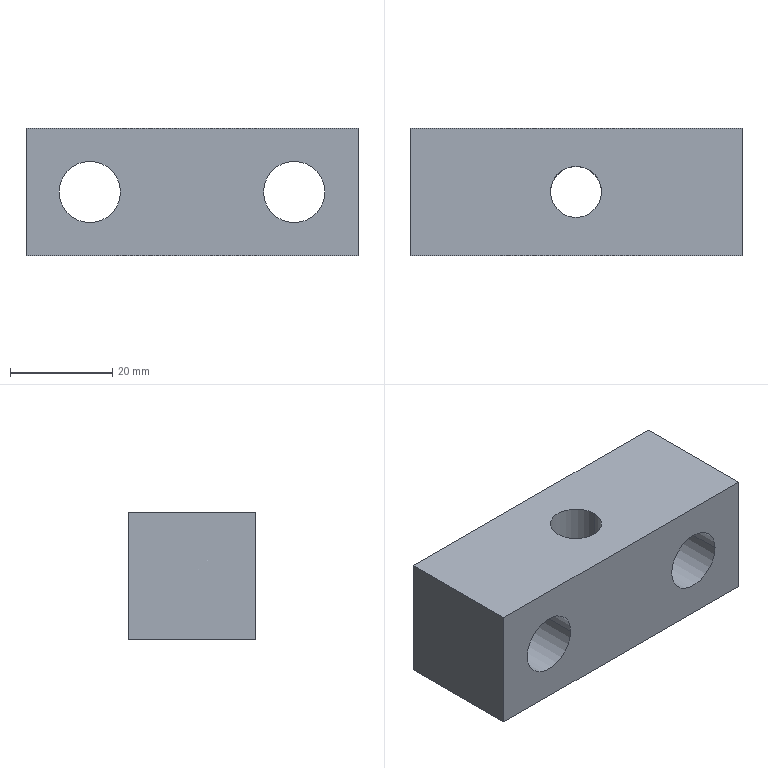Part | STEP file | J452-EBZ05-21-04-Part-1 | 1 solid | 12 faces | box 65 x 25 x 25 mm | volume 33007 mm3 | cylinder 6 | plane 6 | commonest cylinder face diameters 12 x4 10 x2
STEP:
#1=CARTESIAN_POINT('',(0.,0.,0.));
#2=DIRECTION('',(0.,0.,1.));
#3=DIRECTION('',(1.,0.,0.));
#4=AXIS2_PLACEMENT_3D('',#1,#2,#3);
#5=CARTESIAN_POINT('',(27.5,12.5,25.));
#6=VERTEX_POINT('',#5);
#7=CARTESIAN_POINT('',(27.5,12.5,0.));
#8=VERTEX_POINT('',#7);
#9=CARTESIAN_POINT('',(27.5,12.5,25.));
#10=DIRECTION('',(0.,0.,-1.));
#11=VECTOR('',#10,1.);
#12=LINE('',#9,#11);
#13=CARTESIAN_POINT('',(32.5,12.5,25.));
#14=DIRECTION('',(0.,0.,-1.));
#15=DIRECTION('',(-1.,0.,0.));
#16=AXIS2_PLACEMENT_3D('',#13,#14,#15);
#17=CYLINDRICAL_SURFACE('',#16,5.);
#18=CARTESIAN_POINT('',(6.283,0.));
#19=DIRECTION('',(0.,1.));
#20=VECTOR('',#19,1.);
#21=LINE('',#18,#20);
#22=(GEOMETRIC_REPRESENTATION_CONTEXT(2)PARAMETRIC_REPRESENTATION_CONTEXT()REPRESENTATION_CONTEXT('',''));
#23=DEFINITIONAL_REPRESENTATION('',(#21),#22);
#24=PCURVE('',#17,#23);
#25=CARTESIAN_POINT('',(32.5,12.5,25.));
#26=DIRECTION('',(0.,0.,-1.));
#27=DIRECTION('',(-1.,0.,0.));
#28=AXIS2_PLACEMENT_3D('',#25,#26,#27);
#29=CYLINDRICAL_SURFACE('',#28,5.);
#30=CARTESIAN_POINT('',(0.,0.));
#31=DIRECTION('',(0.,1.));
#32=VECTOR('',#31,1.);
#33=LINE('',#30,#32);
#34=(GEOMETRIC_REPRESENTATION_CONTEXT(2)PARAMETRIC_REPRESENTATION_CONTEXT()REPRESENTATION_CONTEXT('',''));
#35=DEFINITIONAL_REPRESENTATION('',(#33),#34);
#36=PCURVE('',#29,#35);
#37=SURFACE_CURVE('',#12,(#24,#36),.PCURVE_S1.);
#38=EDGE_CURVE('',#6,#8,#37,.T.);
#39=ORIENTED_EDGE('',*,*,#38,.T.);
#40=CARTESIAN_POINT('',(37.5,12.5,0.));
#41=VERTEX_POINT('',#40);
#42=CARTESIAN_POINT('',(32.5,12.5,0.));
#43=DIRECTION('',(0.,0.,1.));
#44=DIRECTION('',(1.,0.,0.));
#45=AXIS2_PLACEMENT_3D('',#42,#43,#44);
#46=CIRCLE('',#45,5.);
#47=CARTESIAN_POINT('',(9.425,25.));
#48=DIRECTION('',(-1.,0.));
#49=VECTOR('',#48,1.);
#50=LINE('',#47,#49);
#51=(GEOMETRIC_REPRESENTATION_CONTEXT(2)PARAMETRIC_REPRESENTATION_CONTEXT()REPRESENTATION_CONTEXT('',''));
#52=DEFINITIONAL_REPRESENTATION('',(#50),#51);
#53=PCURVE('',#17,#52);
#54=CARTESIAN_POINT('',(0.,12.5,0.));
#55=DIRECTION('',(0.,0.,-1.));
#56=DIRECTION('',(-1.,0.,0.));
#57=AXIS2_PLACEMENT_3D('',#54,#55,#56);
#58=PLANE('',#57);
#59=CARTESIAN_POINT('',(-37.5,0.));
#60=CARTESIAN_POINT('',(-37.5,8.66));
#61=CARTESIAN_POINT('',(-30.,4.33));
#62=CARTESIAN_POINT('',(-22.5,0.));
#63=CARTESIAN_POINT('',(-30.,-4.33));
#64=CARTESIAN_POINT('',(-37.5,-8.66));
#65=CARTESIAN_POINT('',(-37.5,0.));
#66=(BOUNDED_CURVE()B_SPLINE_CURVE(2,(#59,#60,#61,#62,#63,#64,#65),.UNSPECIFIED.,.T.,.F.)B_SPLINE_CURVE_WITH_KNOTS((1,2,2,2,2,1),(-2.094,0.,2.094,4.189,6.283,8.378),.UNSPECIFIED.)CURVE()GEOMETRIC_REPRESENTATION_ITEM()RATIONAL_B_SPLINE_CURVE((1.,0.5,1.,0.5,1.,0.5,1.))REPRESENTATION_ITEM(''));
#67=(GEOMETRIC_REPRESENTATION_CONTEXT(2)PARAMETRIC_REPRESENTATION_CONTEXT()REPRESENTATION_CONTEXT('',''));
#68=DEFINITIONAL_REPRESENTATION('',(#66),#67);
#69=PCURVE('',#58,#68);
#70=SURFACE_CURVE('',#46,(#53,#69),.PCURVE_S1.);
#71=EDGE_CURVE('',#8,#41,#70,.T.);
#72=ORIENTED_EDGE('',*,*,#71,.T.);
#73=CARTESIAN_POINT('',(37.5,12.5,25.));
#74=VERTEX_POINT('',#73);
#75=CARTESIAN_POINT('',(37.5,12.5,25.));
#76=DIRECTION('',(0.,0.,-1.));
#77=VECTOR('',#76,1.);
#78=LINE('',#75,#77);
#79=CARTESIAN_POINT('',(3.142,0.));
#80=DIRECTION('',(0.,1.));
#81=VECTOR('',#80,1.);
#82=LINE('',#79,#81);
#83=(GEOMETRIC_REPRESENTATION_CONTEXT(2)PARAMETRIC_REPRESENTATION_CONTEXT()REPRESENTATION_CONTEXT('',''));
#84=DEFINITIONAL_REPRESENTATION('',(#82),#83);
#85=PCURVE('',#17,#84);
#86=CARTESIAN_POINT('',(3.142,0.));
#87=DIRECTION('',(0.,1.));
#88=VECTOR('',#87,1.);
#89=LINE('',#86,#88);
#90=(GEOMETRIC_REPRESENTATION_CONTEXT(2)PARAMETRIC_REPRESENTATION_CONTEXT()REPRESENTATION_CONTEXT('',''));
#91=DEFINITIONAL_REPRESENTATION('',(#89),#90);
#92=PCURVE('',#29,#91);
#93=SURFACE_CURVE('',#78,(#85,#92),.PCURVE_S1.);
#94=EDGE_CURVE('',#74,#41,#93,.T.);
#95=ORIENTED_EDGE('',*,*,#94,.F.);
#96=CARTESIAN_POINT('',(32.5,12.5,25.));
#97=DIRECTION('',(0.,0.,-1.));
#98=DIRECTION('',(-1.,0.,0.));
#99=AXIS2_PLACEMENT_3D('',#96,#97,#98);
#100=CIRCLE('',#99,5.);
#101=CARTESIAN_POINT('',(0.,0.));
#102=DIRECTION('',(1.,0.));
#103=VECTOR('',#102,1.);
#104=LINE('',#101,#103);
#105=(GEOMETRIC_REPRESENTATION_CONTEXT(2)PARAMETRIC_REPRESENTATION_CONTEXT()REPRESENTATION_CONTEXT('',''));
#106=DEFINITIONAL_REPRESENTATION('',(#104),#105);
#107=PCURVE('',#17,#106);
#108=CARTESIAN_POINT('',(0.,12.5,25.));
#109=DIRECTION('',(0.,0.,1.));
#110=DIRECTION('',(1.,0.,0.));
#111=AXIS2_PLACEMENT_3D('',#108,#109,#110);
#112=PLANE('',#111);
#113=CARTESIAN_POINT('',(27.5,0.));
#114=CARTESIAN_POINT('',(27.5,8.66));
#115=CARTESIAN_POINT('',(35.,4.33));
#116=CARTESIAN_POINT('',(42.5,0.));
#117=CARTESIAN_POINT('',(35.,-4.33));
#118=CARTESIAN_POINT('',(27.5,-8.66));
#119=CARTESIAN_POINT('',(27.5,0.));
#120=(BOUNDED_CURVE()B_SPLINE_CURVE(2,(#113,#114,#115,#116,#117,#118,#119),.UNSPECIFIED.,.T.,.F.)B_SPLINE_CURVE_WITH_KNOTS((1,2,2,2,2,1),(-2.094,0.,2.094,4.189,6.283,8.378),.UNSPECIFIED.)CURVE()GEOMETRIC_REPRESENTATION_ITEM()RATIONAL_B_SPLINE_CURVE((1.,0.5,1.,0.5,1.,0.5,1.))REPRESENTATION_ITEM(''));
#121=(GEOMETRIC_REPRESENTATION_CONTEXT(2)PARAMETRIC_REPRESENTATION_CONTEXT()REPRESENTATION_CONTEXT('',''));
#122=DEFINITIONAL_REPRESENTATION('',(#120),#121);
#123=PCURVE('',#112,#122);
#124=SURFACE_CURVE('',#100,(#107,#123),.PCURVE_S1.);
#125=EDGE_CURVE('',#74,#6,#124,.T.);
#126=ORIENTED_EDGE('',*,*,#125,.T.);
#127=EDGE_LOOP('',(#39,#72,#95,#126));
#128=FACE_BOUND('',#127,.F.);
#129=ADVANCED_FACE('',(#128),#17,.F.);
#130=CARTESIAN_POINT('',(46.5,0.,12.5));
#131=VERTEX_POINT('',#130);
#132=CARTESIAN_POINT('',(46.5,25.,12.5));
#133=VERTEX_POINT('',#132);
#134=CARTESIAN_POINT('',(46.5,0.,12.5));
#135=DIRECTION('',(0.,1.,0.));
#136=VECTOR('',#135,1.);
#137=LINE('',#134,#136);
#138=CARTESIAN_POINT('',(52.5,0.,12.5));
#139=DIRECTION('',(0.,1.,0.));
#140=DIRECTION('',(-1.,0.,0.));
#141=AXIS2_PLACEMENT_3D('',#138,#139,#140);
#142=CYLINDRICAL_SURFACE('',#141,6.);
#143=CARTESIAN_POINT('',(6.283,0.));
#144=DIRECTION('',(0.,1.));
#145=VECTOR('',#144,1.);
#146=LINE('',#143,#145);
#147=(GEOMETRIC_REPRESENTATION_CONTEXT(2)PARAMETRIC_REPRESENTATION_CONTEXT()REPRESENTATION_CONTEXT('',''));
#148=DEFINITIONAL_REPRESENTATION('',(#146),#147);
#149=PCURVE('',#142,#148);
#150=CARTESIAN_POINT('',(52.5,0.,12.5));
#151=DIRECTION('',(0.,1.,0.));
#152=DIRECTION('',(-1.,0.,0.));
#153=AXIS2_PLACEMENT_3D('',#150,#151,#152);
#154=CYLINDRICAL_SURFACE('',#153,6.);
#155=CARTESIAN_POINT('',(0.,0.));
#156=DIRECTION('',(0.,1.));
#157=VECTOR('',#156,1.);
#158=LINE('',#155,#157);
#159=(GEOMETRIC_REPRESENTATION_CONTEXT(2)PARAMETRIC_REPRESENTATION_CONTEXT()REPRESENTATION_CONTEXT('',''));
#160=DEFINITIONAL_REPRESENTATION('',(#158),#159);
#161=PCURVE('',#154,#160);
#162=SURFACE_CURVE('',#137,(#149,#161),.PCURVE_S1.);
#163=EDGE_CURVE('',#131,#133,#162,.T.);
#164=ORIENTED_EDGE('',*,*,#163,.T.);
#165=CARTESIAN_POINT('',(58.5,25.,12.5));
#166=VERTEX_POINT('',#165);
#167=CARTESIAN_POINT('',(52.5,25.,12.5));
#168=DIRECTION('',(0.,-1.,0.));
#169=DIRECTION('',(1.,0.,0.));
#170=AXIS2_PLACEMENT_3D('',#167,#168,#169);
#171=CIRCLE('',#170,6.);
#172=CARTESIAN_POINT('',(9.425,25.));
#173=DIRECTION('',(-1.,0.));
#174=VECTOR('',#173,1.);
#175=LINE('',#172,#174);
#176=(GEOMETRIC_REPRESENTATION_CONTEXT(2)PARAMETRIC_REPRESENTATION_CONTEXT()REPRESENTATION_CONTEXT('',''));
#177=DEFINITIONAL_REPRESENTATION('',(#175),#176);
#178=PCURVE('',#142,#177);
#179=CARTESIAN_POINT('',(0.,25.,12.5));
#180=DIRECTION('',(0.,1.,0.));
#181=DIRECTION('',(-1.,0.,0.));
#182=AXIS2_PLACEMENT_3D('',#179,#180,#181);
#183=PLANE('',#182);
#184=CARTESIAN_POINT('',(-58.5,0.));
#185=CARTESIAN_POINT('',(-58.5,10.392));
#186=CARTESIAN_POINT('',(-49.5,5.196));
#187=CARTESIAN_POINT('',(-40.5,0.));
#188=CARTESIAN_POINT('',(-49.5,-5.196));
#189=CARTESIAN_POINT('',(-58.5,-10.392));
#190=CARTESIAN_POINT('',(-58.5,0.));
#191=(BOUNDED_CURVE()B_SPLINE_CURVE(2,(#184,#185,#186,#187,#188,#189,#190),.UNSPECIFIED.,.T.,.F.)B_SPLINE_CURVE_WITH_KNOTS((1,2,2,2,2,1),(-2.094,0.,2.094,4.189,6.283,8.378),.UNSPECIFIED.)CURVE()GEOMETRIC_REPRESENTATION_ITEM()RATIONAL_B_SPLINE_CURVE((1.,0.5,1.,0.5,1.,0.5,1.))REPRESENTATION_ITEM(''));
#192=(GEOMETRIC_REPRESENTATION_CONTEXT(2)PARAMETRIC_REPRESENTATION_CONTEXT()REPRESENTATION_CONTEXT('',''));
#193=DEFINITIONAL_REPRESENTATION('',(#191),#192);
#194=PCURVE('',#183,#193);
#195=SURFACE_CURVE('',#171,(#178,#194),.PCURVE_S1.);
#196=EDGE_CURVE('',#133,#166,#195,.T.);
#197=ORIENTED_EDGE('',*,*,#196,.T.);
#198=CARTESIAN_POINT('',(58.5,0.,12.5));
#199=VERTEX_POINT('',#198);
#200=CARTESIAN_POINT('',(58.5,0.,12.5));
#201=DIRECTION('',(0.,1.,0.));
#202=VECTOR('',#201,1.);
#203=LINE('',#200,#202);
#204=CARTESIAN_POINT('',(3.142,0.));
#205=DIRECTION('',(0.,1.));
#206=VECTOR('',#205,1.);
#207=LINE('',#204,#206);
#208=(GEOMETRIC_REPRESENTATION_CONTEXT(2)PARAMETRIC_REPRESENTATION_CONTEXT()REPRESENTATION_CONTEXT('',''));
#209=DEFINITIONAL_REPRESENTATION('',(#207),#208);
#210=PCURVE('',#142,#209);
#211=CARTESIAN_POINT('',(3.142,0.));
#212=DIRECTION('',(0.,1.));
#213=VECTOR('',#212,1.);
#214=LINE('',#211,#213);
#215=(GEOMETRIC_REPRESENTATION_CONTEXT(2)PARAMETRIC_REPRESENTATION_CONTEXT()REPRESENTATION_CONTEXT('',''));
#216=DEFINITIONAL_REPRESENTATION('',(#214),#215);
#217=PCURVE('',#154,#216);
#218=SURFACE_CURVE('',#203,(#210,#217),.PCURVE_S1.);
#219=EDGE_CURVE('',#199,#166,#218,.T.);
#220=ORIENTED_EDGE('',*,*,#219,.F.);
#221=CARTESIAN_POINT('',(52.5,0.,12.5));
#222=DIRECTION('',(0.,1.,0.));
#223=DIRECTION('',(-1.,0.,0.));
#224=AXIS2_PLACEMENT_3D('',#221,#222,#223);
#225=CIRCLE('',#224,6.);
#226=CARTESIAN_POINT('',(0.,0.));
#227=DIRECTION('',(1.,0.));
#228=VECTOR('',#227,1.);
#229=LINE('',#226,#228);
#230=(GEOMETRIC_REPRESENTATION_CONTEXT(2)PARAMETRIC_REPRESENTATION_CONTEXT()REPRESENTATION_CONTEXT('',''));
#231=DEFINITIONAL_REPRESENTATION('',(#229),#230);
#232=PCURVE('',#142,#231);
#233=CARTESIAN_POINT('',(0.,0.,12.5));
#234=DIRECTION('',(0.,-1.,0.));
#235=DIRECTION('',(1.,0.,0.));
#236=AXIS2_PLACEMENT_3D('',#233,#234,#235);
#237=PLANE('',#236);
#238=CARTESIAN_POINT('',(46.5,0.));
#239=CARTESIAN_POINT('',(46.5,10.392));
#240=CARTESIAN_POINT('',(55.5,5.196));
#241=CARTESIAN_POINT('',(64.5,0.));
#242=CARTESIAN_POINT('',(55.5,-5.196));
#243=CARTESIAN_POINT('',(46.5,-10.392));
#244=CARTESIAN_POINT('',(46.5,0.));
#245=(BOUNDED_CURVE()B_SPLINE_CURVE(2,(#238,#239,#240,#241,#242,#243,#244),.UNSPECIFIED.,.T.,.F.)B_SPLINE_CURVE_WITH_KNOTS((1,2,2,2,2,1),(-2.094,0.,2.094,4.189,6.283,8.378),.UNSPECIFIED.)CURVE()GEOMETRIC_REPRESENTATION_ITEM()RATIONAL_B_SPLINE_CURVE((1.,0.5,1.,0.5,1.,0.5,1.))REPRESENTATION_ITEM(''));
#246=(GEOMETRIC_REPRESENTATION_CONTEXT(2)PARAMETRIC_REPRESENTATION_CONTEXT()REPRESENTATION_CONTEXT('',''));
#247=DEFINITIONAL_REPRESENTATION('',(#245),#246);
#248=PCURVE('',#237,#247);
#249=SURFACE_CURVE('',#225,(#232,#248),.PCURVE_S1.);
#250=EDGE_CURVE('',#199,#131,#249,.T.);
#251=ORIENTED_EDGE('',*,*,#250,.T.);
#252=EDGE_LOOP('',(#164,#197,#220,#251));
#253=FACE_BOUND('',#252,.F.);
#254=ADVANCED_FACE('',(#253),#142,.F.);
#255=CARTESIAN_POINT('',(6.5,0.,12.5));
#256=VERTEX_POINT('',#255);
#257=CARTESIAN_POINT('',(6.5,25.,12.5));
#258=VERTEX_POINT('',#257);
#259=CARTESIAN_POINT('',(6.5,0.,12.5));
#260=DIRECTION('',(0.,1.,0.));
#261=VECTOR('',#260,1.);
#262=LINE('',#259,#261);
#263=CARTESIAN_POINT('',(12.5,0.,12.5));
#264=DIRECTION('',(0.,1.,0.));
#265=DIRECTION('',(-1.,0.,0.));
#266=AXIS2_PLACEMENT_3D('',#263,#264,#265);
#267=CYLINDRICAL_SURFACE('',#266,6.);
#268=CARTESIAN_POINT('',(6.283,0.));
#269=DIRECTION('',(0.,1.));
#270=VECTOR('',#269,1.);
#271=LINE('',#268,#270);
#272=(GEOMETRIC_REPRESENTATION_CONTEXT(2)PARAMETRIC_REPRESENTATION_CONTEXT()REPRESENTATION_CONTEXT('',''));
#273=DEFINITIONAL_REPRESENTATION('',(#271),#272);
#274=PCURVE('',#267,#273);
#275=CARTESIAN_POINT('',(12.5,0.,12.5));
#276=DIRECTION('',(0.,1.,0.));
#277=DIRECTION('',(-1.,0.,0.));
#278=AXIS2_PLACEMENT_3D('',#275,#276,#277);
#279=CYLINDRICAL_SURFACE('',#278,6.);
#280=CARTESIAN_POINT('',(0.,0.));
#281=DIRECTION('',(0.,1.));
#282=VECTOR('',#281,1.);
#283=LINE('',#280,#282);
#284=(GEOMETRIC_REPRESENTATION_CONTEXT(2)PARAMETRIC_REPRESENTATION_CONTEXT()REPRESENTATION_CONTEXT('',''));
#285=DEFINITIONAL_REPRESENTATION('',(#283),#284);
#286=PCURVE('',#279,#285);
#287=SURFACE_CURVE('',#262,(#274,#286),.PCURVE_S1.);
#288=EDGE_CURVE('',#256,#258,#287,.T.);
#289=ORIENTED_EDGE('',*,*,#288,.T.);
#290=CARTESIAN_POINT('',(18.5,25.,12.5));
#291=VERTEX_POINT('',#290);
#292=CARTESIAN_POINT('',(12.5,25.,12.5));
#293=DIRECTION('',(0.,-1.,0.));
#294=DIRECTION('',(1.,0.,0.));
#295=AXIS2_PLACEMENT_3D('',#292,#293,#294);
#296=CIRCLE('',#295,6.);
#297=CARTESIAN_POINT('',(9.425,25.));
#298=DIRECTION('',(-1.,0.));
#299=VECTOR('',#298,1.);
#300=LINE('',#297,#299);
#301=(GEOMETRIC_REPRESENTATION_CONTEXT(2)PARAMETRIC_REPRESENTATION_CONTEXT()REPRESENTATION_CONTEXT('',''));
#302=DEFINITIONAL_REPRESENTATION('',(#300),#301);
#303=PCURVE('',#267,#302);
#304=CARTESIAN_POINT('',(-18.5,0.));
#305=CARTESIAN_POINT('',(-18.5,10.392));
#306=CARTESIAN_POINT('',(-9.5,5.196));
#307=CARTESIAN_POINT('',(-0.5,0.));
#308=CARTESIAN_POINT('',(-9.5,-5.196));
#309=CARTESIAN_POINT('',(-18.5,-10.392));
#310=CARTESIAN_POINT('',(-18.5,0.));
#311=(BOUNDED_CURVE()B_SPLINE_CURVE(2,(#304,#305,#306,#307,#308,#309,#310),.UNSPECIFIED.,.T.,.F.)B_SPLINE_CURVE_WITH_KNOTS((1,2,2,2,2,1),(-2.094,0.,2.094,4.189,6.283,8.378),.UNSPECIFIED.)CURVE()GEOMETRIC_REPRESENTATION_ITEM()RATIONAL_B_SPLINE_CURVE((1.,0.5,1.,0.5,1.,0.5,1.))REPRESENTATION_ITEM(''));
#312=(GEOMETRIC_REPRESENTATION_CONTEXT(2)PARAMETRIC_REPRESENTATION_CONTEXT()REPRESENTATION_CONTEXT('',''));
#313=DEFINITIONAL_REPRESENTATION('',(#311),#312);
#314=PCURVE('',#183,#313);
#315=SURFACE_CURVE('',#296,(#303,#314),.PCURVE_S1.);
#316=EDGE_CURVE('',#258,#291,#315,.T.);
#317=ORIENTED_EDGE('',*,*,#316,.T.);
#318=CARTESIAN_POINT('',(18.5,0.,12.5));
#319=VERTEX_POINT('',#318);
#320=CARTESIAN_POINT('',(18.5,0.,12.5));
#321=DIRECTION('',(0.,1.,0.));
#322=VECTOR('',#321,1.);
#323=LINE('',#320,#322);
#324=CARTESIAN_POINT('',(3.142,0.));
#325=DIRECTION('',(0.,1.));
#326=VECTOR('',#325,1.);
#327=LINE('',#324,#326);
#328=(GEOMETRIC_REPRESENTATION_CONTEXT(2)PARAMETRIC_REPRESENTATION_CONTEXT()REPRESENTATION_CONTEXT('',''));
#329=DEFINITIONAL_REPRESENTATION('',(#327),#328);
#330=PCURVE('',#267,#329);
#331=CARTESIAN_POINT('',(3.142,0.));
#332=DIRECTION('',(0.,1.));
#333=VECTOR('',#332,1.);
#334=LINE('',#331,#333);
#335=(GEOMETRIC_REPRESENTATION_CONTEXT(2)PARAMETRIC_REPRESENTATION_CONTEXT()REPRESENTATION_CONTEXT('',''));
#336=DEFINITIONAL_REPRESENTATION('',(#334),#335);
#337=PCURVE('',#279,#336);
#338=SURFACE_CURVE('',#323,(#330,#337),.PCURVE_S1.);
#339=EDGE_CURVE('',#319,#291,#338,.T.);
#340=ORIENTED_EDGE('',*,*,#339,.F.);
#341=CARTESIAN_POINT('',(12.5,0.,12.5));
#342=DIRECTION('',(0.,1.,0.));
#343=DIRECTION('',(-1.,0.,0.));
#344=AXIS2_PLACEMENT_3D('',#341,#342,#343);
#345=CIRCLE('',#344,6.);
#346=CARTESIAN_POINT('',(0.,0.));
#347=DIRECTION('',(1.,0.));
#348=VECTOR('',#347,1.);
#349=LINE('',#346,#348);
#350=(GEOMETRIC_REPRESENTATION_CONTEXT(2)PARAMETRIC_REPRESENTATION_CONTEXT()REPRESENTATION_CONTEXT('',''));
#351=DEFINITIONAL_REPRESENTATION('',(#349),#350);
#352=PCURVE('',#267,#351);
#353=CARTESIAN_POINT('',(6.5,0.));
#354=CARTESIAN_POINT('',(6.5,10.392));
#355=CARTESIAN_POINT('',(15.5,5.196));
#356=CARTESIAN_POINT('',(24.5,0.));
#357=CARTESIAN_POINT('',(15.5,-5.196));
#358=CARTESIAN_POINT('',(6.5,-10.392));
#359=CARTESIAN_POINT('',(6.5,0.));
#360=(BOUNDED_CURVE()B_SPLINE_CURVE(2,(#353,#354,#355,#356,#357,#358,#359),.UNSPECIFIED.,.T.,.F.)B_SPLINE_CURVE_WITH_KNOTS((1,2,2,2,2,1),(-2.094,0.,2.094,4.189,6.283,8.378),.UNSPECIFIED.)CURVE()GEOMETRIC_REPRESENTATION_ITEM()RATIONAL_B_SPLINE_CURVE((1.,0.5,1.,0.5,1.,0.5,1.))REPRESENTATION_ITEM(''));
#361=(GEOMETRIC_REPRESENTATION_CONTEXT(2)PARAMETRIC_REPRESENTATION_CONTEXT()REPRESENTATION_CONTEXT('',''));
#362=DEFINITIONAL_REPRESENTATION('',(#360),#361);
#363=PCURVE('',#237,#362);
#364=SURFACE_CURVE('',#345,(#352,#363),.PCURVE_S1.);
#365=EDGE_CURVE('',#319,#256,#364,.T.);
#366=ORIENTED_EDGE('',*,*,#365,.T.);
#367=EDGE_LOOP('',(#289,#317,#340,#366));
#368=FACE_BOUND('',#367,.F.);
#369=ADVANCED_FACE('',(#368),#267,.F.);
#370=CARTESIAN_POINT('',(65.,25.,0.));
#371=VERTEX_POINT('',#370);
#372=CARTESIAN_POINT('',(65.,0.,0.));
#373=VERTEX_POINT('',#372);
#374=CARTESIAN_POINT('',(65.,12.5,0.));
#375=DIRECTION('',(0.,-1.,0.));
#376=VECTOR('',#375,1.);
#377=LINE('',#374,#376);
#378=CARTESIAN_POINT('',(65.,12.5,12.5));
#379=DIRECTION('',(1.,0.,0.));
#380=DIRECTION('',(0.,1.,0.));
#381=AXIS2_PLACEMENT_3D('',#378,#379,#380);
#382=PLANE('',#381);
#383=CARTESIAN_POINT('',(0.,-12.5));
#384=DIRECTION('',(-1.,0.));
#385=VECTOR('',#384,1.);
#386=LINE('',#383,#385);
#387=(GEOMETRIC_REPRESENTATION_CONTEXT(2)PARAMETRIC_REPRESENTATION_CONTEXT()REPRESENTATION_CONTEXT('',''));
#388=DEFINITIONAL_REPRESENTATION('',(#386),#387);
#389=PCURVE('',#382,#388);
#390=CARTESIAN_POINT('',(-65.,0.));
#391=DIRECTION('',(0.,-1.));
#392=VECTOR('',#391,1.);
#393=LINE('',#390,#392);
#394=(GEOMETRIC_REPRESENTATION_CONTEXT(2)PARAMETRIC_REPRESENTATION_CONTEXT()REPRESENTATION_CONTEXT('',''));
#395=DEFINITIONAL_REPRESENTATION('',(#393),#394);
#396=PCURVE('',#58,#395);
#397=SURFACE_CURVE('',#377,(#389,#396),.PCURVE_S1.);
#398=EDGE_CURVE('',#371,#373,#397,.T.);
#399=ORIENTED_EDGE('',*,*,#398,.F.);
#400=CARTESIAN_POINT('',(65.,25.,25.));
#401=VERTEX_POINT('',#400);
#402=CARTESIAN_POINT('',(65.,25.,12.5));
#403=DIRECTION('',(0.,0.,-1.));
#404=VECTOR('',#403,1.);
#405=LINE('',#402,#404);
#406=CARTESIAN_POINT('',(12.5,0.));
#407=DIRECTION('',(0.,-1.));
#408=VECTOR('',#407,1.);
#409=LINE('',#406,#408);
#410=(GEOMETRIC_REPRESENTATION_CONTEXT(2)PARAMETRIC_REPRESENTATION_CONTEXT()REPRESENTATION_CONTEXT('',''));
#411=DEFINITIONAL_REPRESENTATION('',(#409),#410);
#412=PCURVE('',#382,#411);
#413=CARTESIAN_POINT('',(-65.,0.));
#414=DIRECTION('',(0.,-1.));
#415=VECTOR('',#414,1.);
#416=LINE('',#413,#415);
#417=(GEOMETRIC_REPRESENTATION_CONTEXT(2)PARAMETRIC_REPRESENTATION_CONTEXT()REPRESENTATION_CONTEXT('',''));
#418=DEFINITIONAL_REPRESENTATION('',(#416),#417);
#419=PCURVE('',#183,#418);
#420=SURFACE_CURVE('',#405,(#412,#419),.PCURVE_S1.);
#421=EDGE_CURVE('',#401,#371,#420,.T.);
#422=ORIENTED_EDGE('',*,*,#421,.F.);
#423=CARTESIAN_POINT('',(65.,0.,25.));
#424=VERTEX_POINT('',#423);
#425=CARTESIAN_POINT('',(65.,12.5,25.));
#426=DIRECTION('',(0.,1.,0.));
#427=VECTOR('',#426,1.);
#428=LINE('',#425,#427);
#429=CARTESIAN_POINT('',(0.,12.5));
#430=DIRECTION('',(1.,0.));
#431=VECTOR('',#430,1.);
#432=LINE('',#429,#431);
#433=(GEOMETRIC_REPRESENTATION_CONTEXT(2)PARAMETRIC_REPRESENTATION_CONTEXT()REPRESENTATION_CONTEXT('',''));
#434=DEFINITIONAL_REPRESENTATION('',(#432),#433);
#435=PCURVE('',#382,#434);
#436=CARTESIAN_POINT('',(65.,0.));
#437=DIRECTION('',(0.,1.));
#438=VECTOR('',#437,1.);
#439=LINE('',#436,#438);
#440=(GEOMETRIC_REPRESENTATION_CONTEXT(2)PARAMETRIC_REPRESENTATION_CONTEXT()REPRESENTATION_CONTEXT('',''));
#441=DEFINITIONAL_REPRESENTATION('',(#439),#440);
#442=PCURVE('',#112,#441);
#443=SURFACE_CURVE('',#428,(#435,#442),.PCURVE_S1.);
#444=EDGE_CURVE('',#424,#401,#443,.T.);
#445=ORIENTED_EDGE('',*,*,#444,.F.);
#446=CARTESIAN_POINT('',(65.,0.,12.5));
#447=DIRECTION('',(0.,0.,1.));
#448=VECTOR('',#447,1.);
#449=LINE('',#446,#448);
#450=CARTESIAN_POINT('',(-12.5,0.));
#451=DIRECTION('',(0.,1.));
#452=VECTOR('',#451,1.);
#453=LINE('',#450,#452);
#454=(GEOMETRIC_REPRESENTATION_CONTEXT(2)PARAMETRIC_REPRESENTATION_CONTEXT()REPRESENTATION_CONTEXT('',''));
#455=DEFINITIONAL_REPRESENTATION('',(#453),#454);
#456=PCURVE('',#382,#455);
#457=CARTESIAN_POINT('',(65.,0.));
#458=DIRECTION('',(0.,1.));
#459=VECTOR('',#458,1.);
#460=LINE('',#457,#459);
#461=(GEOMETRIC_REPRESENTATION_CONTEXT(2)PARAMETRIC_REPRESENTATION_CONTEXT()REPRESENTATION_CONTEXT('',''));
#462=DEFINITIONAL_REPRESENTATION('',(#460),#461);
#463=PCURVE('',#237,#462);
#464=SURFACE_CURVE('',#449,(#456,#463),.PCURVE_S1.);
#465=EDGE_CURVE('',#373,#424,#464,.T.);
#466=ORIENTED_EDGE('',*,*,#465,.F.);
#467=EDGE_LOOP('',(#399,#422,#445,#466));
#468=FACE_BOUND('',#467,.T.);
#469=ADVANCED_FACE('',(#468),#382,.T.);
#470=ORIENTED_EDGE('',*,*,#71,.T.);
#471=CARTESIAN_POINT('',(32.5,12.5,0.));
#472=DIRECTION('',(0.,0.,1.));
#473=DIRECTION('',(1.,0.,0.));
#474=AXIS2_PLACEMENT_3D('',#471,#472,#473);
#475=CIRCLE('',#474,5.);
#476=CARTESIAN_POINT('',(-37.5,0.));
#477=CARTESIAN_POINT('',(-37.5,8.66));
#478=CARTESIAN_POINT('',(-30.,4.33));
#479=CARTESIAN_POINT('',(-22.5,0.));
#480=CARTESIAN_POINT('',(-30.,-4.33));
#481=CARTESIAN_POINT('',(-37.5,-8.66));
#482=CARTESIAN_POINT('',(-37.5,0.));
#483=(BOUNDED_CURVE()B_SPLINE_CURVE(2,(#476,#477,#478,#479,#480,#481,#482),.UNSPECIFIED.,.T.,.F.)B_SPLINE_CURVE_WITH_KNOTS((1,2,2,2,2,1),(-2.094,0.,2.094,4.189,6.283,8.378),.UNSPECIFIED.)CURVE()GEOMETRIC_REPRESENTATION_ITEM()RATIONAL_B_SPLINE_CURVE((1.,0.5,1.,0.5,1.,0.5,1.))REPRESENTATION_ITEM(''));
#484=(GEOMETRIC_REPRESENTATION_CONTEXT(2)PARAMETRIC_REPRESENTATION_CONTEXT()REPRESENTATION_CONTEXT('',''));
#485=DEFINITIONAL_REPRESENTATION('',(#483),#484);
#486=PCURVE('',#58,#485);
#487=CARTESIAN_POINT('',(3.142,25.));
#488=DIRECTION('',(-1.,0.));
#489=VECTOR('',#488,1.);
#490=LINE('',#487,#489);
#491=(GEOMETRIC_REPRESENTATION_CONTEXT(2)PARAMETRIC_REPRESENTATION_CONTEXT()REPRESENTATION_CONTEXT('',''));
#492=DEFINITIONAL_REPRESENTATION('',(#490),#491);
#493=PCURVE('',#29,#492);
#494=SURFACE_CURVE('',#475,(#486,#493),.PCURVE_S1.);
#495=EDGE_CURVE('',#41,#8,#494,.T.);
#496=ORIENTED_EDGE('',*,*,#495,.T.);
#497=EDGE_LOOP('',(#470,#496));
#498=FACE_BOUND('',#497,.T.);
#499=CARTESIAN_POINT('',(0.,25.,0.));
#500=VERTEX_POINT('',#499);
#501=CARTESIAN_POINT('',(0.,25.,0.));
#502=DIRECTION('',(1.,0.,0.));
#503=VECTOR('',#502,1.);
#504=LINE('',#501,#503);
#505=CARTESIAN_POINT('',(0.,12.5));
#506=DIRECTION('',(-1.,0.));
#507=VECTOR('',#506,1.);
#508=LINE('',#505,#507);
#509=(GEOMETRIC_REPRESENTATION_CONTEXT(2)PARAMETRIC_REPRESENTATION_CONTEXT()REPRESENTATION_CONTEXT('',''));
#510=DEFINITIONAL_REPRESENTATION('',(#508),#509);
#511=PCURVE('',#58,#510);
#512=CARTESIAN_POINT('',(0.,-12.5));
#513=DIRECTION('',(-1.,0.));
#514=VECTOR('',#513,1.);
#515=LINE('',#512,#514);
#516=(GEOMETRIC_REPRESENTATION_CONTEXT(2)PARAMETRIC_REPRESENTATION_CONTEXT()REPRESENTATION_CONTEXT('',''));
#517=DEFINITIONAL_REPRESENTATION('',(#515),#516);
#518=PCURVE('',#183,#517);
#519=SURFACE_CURVE('',#504,(#511,#518),.PCURVE_S1.);
#520=EDGE_CURVE('',#500,#371,#519,.T.);
#521=ORIENTED_EDGE('',*,*,#520,.T.);
#522=ORIENTED_EDGE('',*,*,#398,.T.);
#523=CARTESIAN_POINT('',(0.,0.,0.));
#524=VERTEX_POINT('',#523);
#525=CARTESIAN_POINT('',(0.,0.,0.));
#526=DIRECTION('',(1.,0.,0.));
#527=VECTOR('',#526,1.);
#528=LINE('',#525,#527);
#529=CARTESIAN_POINT('',(0.,-12.5));
#530=DIRECTION('',(-1.,0.));
#531=VECTOR('',#530,1.);
#532=LINE('',#529,#531);
#533=(GEOMETRIC_REPRESENTATION_CONTEXT(2)PARAMETRIC_REPRESENTATION_CONTEXT()REPRESENTATION_CONTEXT('',''));
#534=DEFINITIONAL_REPRESENTATION('',(#532),#533);
#535=PCURVE('',#58,#534);
#536=CARTESIAN_POINT('',(0.,-12.5));
#537=DIRECTION('',(1.,0.));
#538=VECTOR('',#537,1.);
#539=LINE('',#536,#538);
#540=(GEOMETRIC_REPRESENTATION_CONTEXT(2)PARAMETRIC_REPRESENTATION_CONTEXT()REPRESENTATION_CONTEXT('',''));
#541=DEFINITIONAL_REPRESENTATION('',(#539),#540);
#542=PCURVE('',#237,#541);
#543=SURFACE_CURVE('',#528,(#535,#542),.PCURVE_S1.);
#544=EDGE_CURVE('',#524,#373,#543,.T.);
#545=ORIENTED_EDGE('',*,*,#544,.F.);
#546=CARTESIAN_POINT('',(0.,12.5,0.));
#547=DIRECTION('',(0.,1.,0.));
#548=VECTOR('',#547,1.);
#549=LINE('',#546,#548);
#550=CARTESIAN_POINT('',(0.,0.));
#551=DIRECTION('',(0.,1.));
#552=VECTOR('',#551,1.);
#553=LINE('',#550,#552);
#554=(GEOMETRIC_REPRESENTATION_CONTEXT(2)PARAMETRIC_REPRESENTATION_CONTEXT()REPRESENTATION_CONTEXT('',''));
#555=DEFINITIONAL_REPRESENTATION('',(#553),#554);
#556=PCURVE('',#58,#555);
#557=CARTESIAN_POINT('',(0.,12.5,12.5));
#558=DIRECTION('',(-1.,0.,0.));
#559=DIRECTION('',(0.,-1.,0.));
#560=AXIS2_PLACEMENT_3D('',#557,#558,#559);
#561=PLANE('',#560);
#562=CARTESIAN_POINT('',(0.,-12.5));
#563=DIRECTION('',(-1.,0.));
#564=VECTOR('',#563,1.);
#565=LINE('',#562,#564);
#566=(GEOMETRIC_REPRESENTATION_CONTEXT(2)PARAMETRIC_REPRESENTATION_CONTEXT()REPRESENTATION_CONTEXT('',''));
#567=DEFINITIONAL_REPRESENTATION('',(#565),#566);
#568=PCURVE('',#561,#567);
#569=SURFACE_CURVE('',#549,(#556,#568),.PCURVE_S1.);
#570=EDGE_CURVE('',#524,#500,#569,.T.);
#571=ORIENTED_EDGE('',*,*,#570,.T.);
#572=EDGE_LOOP('',(#521,#522,#545,#571));
#573=FACE_BOUND('',#572,.T.);
#574=ADVANCED_FACE('',(#498,#573),#58,.T.);
#575=CARTESIAN_POINT('',(52.5,0.,12.5));
#576=DIRECTION('',(0.,1.,0.));
#577=DIRECTION('',(-1.,0.,0.));
#578=AXIS2_PLACEMENT_3D('',#575,#576,#577);
#579=CIRCLE('',#578,6.);
#580=CARTESIAN_POINT('',(46.5,0.));
#581=CARTESIAN_POINT('',(46.5,10.392));
#582=CARTESIAN_POINT('',(55.5,5.196));
#583=CARTESIAN_POINT('',(64.5,0.));
#584=CARTESIAN_POINT('',(55.5,-5.196));
#585=CARTESIAN_POINT('',(46.5,-10.392));
#586=CARTESIAN_POINT('',(46.5,0.));
#587=(BOUNDED_CURVE()B_SPLINE_CURVE(2,(#580,#581,#582,#583,#584,#585,#586),.UNSPECIFIED.,.T.,.F.)B_SPLINE_CURVE_WITH_KNOTS((1,2,2,2,2,1),(-2.094,0.,2.094,4.189,6.283,8.378),.UNSPECIFIED.)CURVE()GEOMETRIC_REPRESENTATION_ITEM()RATIONAL_B_SPLINE_CURVE((1.,0.5,1.,0.5,1.,0.5,1.))REPRESENTATION_ITEM(''));
#588=(GEOMETRIC_REPRESENTATION_CONTEXT(2)PARAMETRIC_REPRESENTATION_CONTEXT()REPRESENTATION_CONTEXT('',''));
#589=DEFINITIONAL_REPRESENTATION('',(#587),#588);
#590=PCURVE('',#237,#589);
#591=CARTESIAN_POINT('',(0.,0.));
#592=DIRECTION('',(1.,0.));
#593=VECTOR('',#592,1.);
#594=LINE('',#591,#593);
#595=(GEOMETRIC_REPRESENTATION_CONTEXT(2)PARAMETRIC_REPRESENTATION_CONTEXT()REPRESENTATION_CONTEXT('',''));
#596=DEFINITIONAL_REPRESENTATION('',(#594),#595);
#597=PCURVE('',#154,#596);
#598=SURFACE_CURVE('',#579,(#590,#597),.PCURVE_S1.);
#599=EDGE_CURVE('',#131,#199,#598,.T.);
#600=ORIENTED_EDGE('',*,*,#599,.T.);
#601=ORIENTED_EDGE('',*,*,#250,.T.);
#602=EDGE_LOOP('',(#600,#601));
#603=FACE_BOUND('',#602,.T.);
#604=CARTESIAN_POINT('',(12.5,0.,12.5));
#605=DIRECTION('',(0.,1.,0.));
#606=DIRECTION('',(-1.,0.,0.));
#607=AXIS2_PLACEMENT_3D('',#604,#605,#606);
#608=CIRCLE('',#607,6.);
#609=CARTESIAN_POINT('',(6.5,0.));
#610=CARTESIAN_POINT('',(6.5,10.392));
#611=CARTESIAN_POINT('',(15.5,5.196));
#612=CARTESIAN_POINT('',(24.5,0.));
#613=CARTESIAN_POINT('',(15.5,-5.196));
#614=CARTESIAN_POINT('',(6.5,-10.392));
#615=CARTESIAN_POINT('',(6.5,0.));
#616=(BOUNDED_CURVE()B_SPLINE_CURVE(2,(#609,#610,#611,#612,#613,#614,#615),.UNSPECIFIED.,.T.,.F.)B_SPLINE_CURVE_WITH_KNOTS((1,2,2,2,2,1),(-2.094,0.,2.094,4.189,6.283,8.378),.UNSPECIFIED.)CURVE()GEOMETRIC_REPRESENTATION_ITEM()RATIONAL_B_SPLINE_CURVE((1.,0.5,1.,0.5,1.,0.5,1.))REPRESENTATION_ITEM(''));
#617=(GEOMETRIC_REPRESENTATION_CONTEXT(2)PARAMETRIC_REPRESENTATION_CONTEXT()REPRESENTATION_CONTEXT('',''));
#618=DEFINITIONAL_REPRESENTATION('',(#616),#617);
#619=PCURVE('',#237,#618);
#620=CARTESIAN_POINT('',(0.,0.));
#621=DIRECTION('',(1.,0.));
#622=VECTOR('',#621,1.);
#623=LINE('',#620,#622);
#624=(GEOMETRIC_REPRESENTATION_CONTEXT(2)PARAMETRIC_REPRESENTATION_CONTEXT()REPRESENTATION_CONTEXT('',''));
#625=DEFINITIONAL_REPRESENTATION('',(#623),#624);
#626=PCURVE('',#279,#625);
#627=SURFACE_CURVE('',#608,(#619,#626),.PCURVE_S1.);
#628=EDGE_CURVE('',#256,#319,#627,.T.);
#629=ORIENTED_EDGE('',*,*,#628,.T.);
#630=ORIENTED_EDGE('',*,*,#365,.T.);
#631=EDGE_LOOP('',(#629,#630));
#632=FACE_BOUND('',#631,.T.);
#633=ORIENTED_EDGE('',*,*,#544,.T.);
#634=ORIENTED_EDGE('',*,*,#465,.T.);
#635=CARTESIAN_POINT('',(0.,0.,25.));
#636=VERTEX_POINT('',#635);
#637=CARTESIAN_POINT('',(0.,0.,25.));
#638=DIRECTION('',(1.,0.,0.));
#639=VECTOR('',#638,1.);
#640=LINE('',#637,#639);
#641=CARTESIAN_POINT('',(0.,12.5));
#642=DIRECTION('',(1.,0.));
#643=VECTOR('',#642,1.);
#644=LINE('',#641,#643);
#645=(GEOMETRIC_REPRESENTATION_CONTEXT(2)PARAMETRIC_REPRESENTATION_CONTEXT()REPRESENTATION_CONTEXT('',''));
#646=DEFINITIONAL_REPRESENTATION('',(#644),#645);
#647=PCURVE('',#237,#646);
#648=CARTESIAN_POINT('',(0.,-12.5));
#649=DIRECTION('',(1.,0.));
#650=VECTOR('',#649,1.);
#651=LINE('',#648,#650);
#652=(GEOMETRIC_REPRESENTATION_CONTEXT(2)PARAMETRIC_REPRESENTATION_CONTEXT()REPRESENTATION_CONTEXT('',''));
#653=DEFINITIONAL_REPRESENTATION('',(#651),#652);
#654=PCURVE('',#112,#653);
#655=SURFACE_CURVE('',#640,(#647,#654),.PCURVE_S1.);
#656=EDGE_CURVE('',#636,#424,#655,.T.);
#657=ORIENTED_EDGE('',*,*,#656,.F.);
#658=CARTESIAN_POINT('',(0.,0.,12.5));
#659=DIRECTION('',(0.,0.,-1.));
#660=VECTOR('',#659,1.);
#661=LINE('',#658,#660);
#662=CARTESIAN_POINT('',(0.,0.));
#663=DIRECTION('',(0.,-1.));
#664=VECTOR('',#663,1.);
#665=LINE('',#662,#664);
#666=(GEOMETRIC_REPRESENTATION_CONTEXT(2)PARAMETRIC_REPRESENTATION_CONTEXT()REPRESENTATION_CONTEXT('',''));
#667=DEFINITIONAL_REPRESENTATION('',(#665),#666);
#668=PCURVE('',#237,#667);
#669=CARTESIAN_POINT('',(12.5,0.));
#670=DIRECTION('',(0.,-1.));
#671=VECTOR('',#670,1.);
#672=LINE('',#669,#671);
#673=(GEOMETRIC_REPRESENTATION_CONTEXT(2)PARAMETRIC_REPRESENTATION_CONTEXT()REPRESENTATION_CONTEXT('',''));
#674=DEFINITIONAL_REPRESENTATION('',(#672),#673);
#675=PCURVE('',#561,#674);
#676=SURFACE_CURVE('',#661,(#668,#675),.PCURVE_S1.);
#677=EDGE_CURVE('',#636,#524,#676,.T.);
#678=ORIENTED_EDGE('',*,*,#677,.T.);
#679=EDGE_LOOP('',(#633,#634,#657,#678));
#680=FACE_BOUND('',#679,.T.);
#681=ADVANCED_FACE('',(#603,#632,#680),#237,.T.);
#682=CARTESIAN_POINT('',(32.5,12.5,25.));
#683=DIRECTION('',(0.,0.,-1.));
#684=DIRECTION('',(-1.,0.,0.));
#685=AXIS2_PLACEMENT_3D('',#682,#683,#684);
#686=CIRCLE('',#685,5.);
#687=CARTESIAN_POINT('',(27.5,0.));
#688=CARTESIAN_POINT('',(27.5,8.66));
#689=CARTESIAN_POINT('',(35.,4.33));
#690=CARTESIAN_POINT('',(42.5,0.));
#691=CARTESIAN_POINT('',(35.,-4.33));
#692=CARTESIAN_POINT('',(27.5,-8.66));
#693=CARTESIAN_POINT('',(27.5,0.));
#694=(BOUNDED_CURVE()B_SPLINE_CURVE(2,(#687,#688,#689,#690,#691,#692,#693),.UNSPECIFIED.,.T.,.F.)B_SPLINE_CURVE_WITH_KNOTS((1,2,2,2,2,1),(-2.094,0.,2.094,4.189,6.283,8.378),.UNSPECIFIED.)CURVE()GEOMETRIC_REPRESENTATION_ITEM()RATIONAL_B_SPLINE_CURVE((1.,0.5,1.,0.5,1.,0.5,1.))REPRESENTATION_ITEM(''));
#695=(GEOMETRIC_REPRESENTATION_CONTEXT(2)PARAMETRIC_REPRESENTATION_CONTEXT()REPRESENTATION_CONTEXT('',''));
#696=DEFINITIONAL_REPRESENTATION('',(#694),#695);
#697=PCURVE('',#112,#696);
#698=CARTESIAN_POINT('',(0.,0.));
#699=DIRECTION('',(1.,0.));
#700=VECTOR('',#699,1.);
#701=LINE('',#698,#700);
#702=(GEOMETRIC_REPRESENTATION_CONTEXT(2)PARAMETRIC_REPRESENTATION_CONTEXT()REPRESENTATION_CONTEXT('',''));
#703=DEFINITIONAL_REPRESENTATION('',(#701),#702);
#704=PCURVE('',#29,#703);
#705=SURFACE_CURVE('',#686,(#697,#704),.PCURVE_S1.);
#706=EDGE_CURVE('',#6,#74,#705,.T.);
#707=ORIENTED_EDGE('',*,*,#706,.T.);
#708=ORIENTED_EDGE('',*,*,#125,.T.);
#709=EDGE_LOOP('',(#707,#708));
#710=FACE_BOUND('',#709,.T.);
#711=ORIENTED_EDGE('',*,*,#656,.T.);
#712=ORIENTED_EDGE('',*,*,#444,.T.);
#713=CARTESIAN_POINT('',(0.,25.,25.));
#714=VERTEX_POINT('',#713);
#715=CARTESIAN_POINT('',(0.,25.,25.));
#716=DIRECTION('',(1.,0.,0.));
#717=VECTOR('',#716,1.);
#718=LINE('',#715,#717);
#719=CARTESIAN_POINT('',(0.,12.5));
#720=DIRECTION('',(1.,0.));
#721=VECTOR('',#720,1.);
#722=LINE('',#719,#721);
#723=(GEOMETRIC_REPRESENTATION_CONTEXT(2)PARAMETRIC_REPRESENTATION_CONTEXT()REPRESENTATION_CONTEXT('',''));
#724=DEFINITIONAL_REPRESENTATION('',(#722),#723);
#725=PCURVE('',#112,#724);
#726=CARTESIAN_POINT('',(0.,12.5));
#727=DIRECTION('',(-1.,0.));
#728=VECTOR('',#727,1.);
#729=LINE('',#726,#728);
#730=(GEOMETRIC_REPRESENTATION_CONTEXT(2)PARAMETRIC_REPRESENTATION_CONTEXT()REPRESENTATION_CONTEXT('',''));
#731=DEFINITIONAL_REPRESENTATION('',(#729),#730);
#732=PCURVE('',#183,#731);
#733=SURFACE_CURVE('',#718,(#725,#732),.PCURVE_S1.);
#734=EDGE_CURVE('',#714,#401,#733,.T.);
#735=ORIENTED_EDGE('',*,*,#734,.F.);
#736=CARTESIAN_POINT('',(0.,12.5,25.));
#737=DIRECTION('',(0.,-1.,0.));
#738=VECTOR('',#737,1.);
#739=LINE('',#736,#738);
#740=CARTESIAN_POINT('',(0.,0.));
#741=DIRECTION('',(0.,-1.));
#742=VECTOR('',#741,1.);
#743=LINE('',#740,#742);
#744=(GEOMETRIC_REPRESENTATION_CONTEXT(2)PARAMETRIC_REPRESENTATION_CONTEXT()REPRESENTATION_CONTEXT('',''));
#745=DEFINITIONAL_REPRESENTATION('',(#743),#744);
#746=PCURVE('',#112,#745);
#747=CARTESIAN_POINT('',(0.,12.5));
#748=DIRECTION('',(1.,0.));
#749=VECTOR('',#748,1.);
#750=LINE('',#747,#749);
#751=(GEOMETRIC_REPRESENTATION_CONTEXT(2)PARAMETRIC_REPRESENTATION_CONTEXT()REPRESENTATION_CONTEXT('',''));
#752=DEFINITIONAL_REPRESENTATION('',(#750),#751);
#753=PCURVE('',#561,#752);
#754=SURFACE_CURVE('',#739,(#746,#753),.PCURVE_S1.);
#755=EDGE_CURVE('',#714,#636,#754,.T.);
#756=ORIENTED_EDGE('',*,*,#755,.T.);
#757=EDGE_LOOP('',(#711,#712,#735,#756));
#758=FACE_BOUND('',#757,.T.);
#759=ADVANCED_FACE('',(#710,#758),#112,.T.);
#760=CARTESIAN_POINT('',(0.,25.,12.5));
#761=DIRECTION('',(0.,0.,1.));
#762=VECTOR('',#761,1.);
#763=LINE('',#760,#762);
#764=CARTESIAN_POINT('',(-12.5,0.));
#765=DIRECTION('',(0.,1.));
#766=VECTOR('',#765,1.);
#767=LINE('',#764,#766);
#768=(GEOMETRIC_REPRESENTATION_CONTEXT(2)PARAMETRIC_REPRESENTATION_CONTEXT()REPRESENTATION_CONTEXT('',''));
#769=DEFINITIONAL_REPRESENTATION('',(#767),#768);
#770=PCURVE('',#561,#769);
#771=CARTESIAN_POINT('',(0.,0.));
#772=DIRECTION('',(0.,1.));
#773=VECTOR('',#772,1.);
#774=LINE('',#771,#773);
#775=(GEOMETRIC_REPRESENTATION_CONTEXT(2)PARAMETRIC_REPRESENTATION_CONTEXT()REPRESENTATION_CONTEXT('',''));
#776=DEFINITIONAL_REPRESENTATION('',(#774),#775);
#777=PCURVE('',#183,#776);
#778=SURFACE_CURVE('',#763,(#770,#777),.PCURVE_S1.);
#779=EDGE_CURVE('',#500,#714,#778,.T.);
#780=ORIENTED_EDGE('',*,*,#779,.F.);
#781=ORIENTED_EDGE('',*,*,#570,.F.);
#782=ORIENTED_EDGE('',*,*,#677,.F.);
#783=ORIENTED_EDGE('',*,*,#755,.F.);
#784=EDGE_LOOP('',(#780,#781,#782,#783));
#785=FACE_BOUND('',#784,.T.);
#786=ADVANCED_FACE('',(#785),#561,.T.);
#787=ORIENTED_EDGE('',*,*,#196,.T.);
#788=CARTESIAN_POINT('',(52.5,25.,12.5));
#789=DIRECTION('',(0.,-1.,0.));
#790=DIRECTION('',(1.,0.,0.));
#791=AXIS2_PLACEMENT_3D('',#788,#789,#790);
#792=CIRCLE('',#791,6.);
#793=CARTESIAN_POINT('',(-58.5,0.));
#794=CARTESIAN_POINT('',(-58.5,10.392));
#795=CARTESIAN_POINT('',(-49.5,5.196));
#796=CARTESIAN_POINT('',(-40.5,0.));
#797=CARTESIAN_POINT('',(-49.5,-5.196));
#798=CARTESIAN_POINT('',(-58.5,-10.392));
#799=CARTESIAN_POINT('',(-58.5,0.));
#800=(BOUNDED_CURVE()B_SPLINE_CURVE(2,(#793,#794,#795,#796,#797,#798,#799),.UNSPECIFIED.,.T.,.F.)B_SPLINE_CURVE_WITH_KNOTS((1,2,2,2,2,1),(-2.094,0.,2.094,4.189,6.283,8.378),.UNSPECIFIED.)CURVE()GEOMETRIC_REPRESENTATION_ITEM()RATIONAL_B_SPLINE_CURVE((1.,0.5,1.,0.5,1.,0.5,1.))REPRESENTATION_ITEM(''));
#801=(GEOMETRIC_REPRESENTATION_CONTEXT(2)PARAMETRIC_REPRESENTATION_CONTEXT()REPRESENTATION_CONTEXT('',''));
#802=DEFINITIONAL_REPRESENTATION('',(#800),#801);
#803=PCURVE('',#183,#802);
#804=CARTESIAN_POINT('',(3.142,25.));
#805=DIRECTION('',(-1.,0.));
#806=VECTOR('',#805,1.);
#807=LINE('',#804,#806);
#808=(GEOMETRIC_REPRESENTATION_CONTEXT(2)PARAMETRIC_REPRESENTATION_CONTEXT()REPRESENTATION_CONTEXT('',''));
#809=DEFINITIONAL_REPRESENTATION('',(#807),#808);
#810=PCURVE('',#154,#809);
#811=SURFACE_CURVE('',#792,(#803,#810),.PCURVE_S1.);
#812=EDGE_CURVE('',#166,#133,#811,.T.);
#813=ORIENTED_EDGE('',*,*,#812,.T.);
#814=EDGE_LOOP('',(#787,#813));
#815=FACE_BOUND('',#814,.T.);
#816=ORIENTED_EDGE('',*,*,#316,.T.);
#817=CARTESIAN_POINT('',(12.5,25.,12.5));
#818=DIRECTION('',(0.,-1.,0.));
#819=DIRECTION('',(1.,0.,0.));
#820=AXIS2_PLACEMENT_3D('',#817,#818,#819);
#821=CIRCLE('',#820,6.);
#822=CARTESIAN_POINT('',(-18.5,0.));
#823=CARTESIAN_POINT('',(-18.5,10.392));
#824=CARTESIAN_POINT('',(-9.5,5.196));
#825=CARTESIAN_POINT('',(-0.5,0.));
#826=CARTESIAN_POINT('',(-9.5,-5.196));
#827=CARTESIAN_POINT('',(-18.5,-10.392));
#828=CARTESIAN_POINT('',(-18.5,0.));
#829=(BOUNDED_CURVE()B_SPLINE_CURVE(2,(#822,#823,#824,#825,#826,#827,#828),.UNSPECIFIED.,.T.,.F.)B_SPLINE_CURVE_WITH_KNOTS((1,2,2,2,2,1),(-2.094,0.,2.094,4.189,6.283,8.378),.UNSPECIFIED.)CURVE()GEOMETRIC_REPRESENTATION_ITEM()RATIONAL_B_SPLINE_CURVE((1.,0.5,1.,0.5,1.,0.5,1.))REPRESENTATION_ITEM(''));
#830=(GEOMETRIC_REPRESENTATION_CONTEXT(2)PARAMETRIC_REPRESENTATION_CONTEXT()REPRESENTATION_CONTEXT('',''));
#831=DEFINITIONAL_REPRESENTATION('',(#829),#830);
#832=PCURVE('',#183,#831);
#833=CARTESIAN_POINT('',(3.142,25.));
#834=DIRECTION('',(-1.,0.));
#835=VECTOR('',#834,1.);
#836=LINE('',#833,#835);
#837=(GEOMETRIC_REPRESENTATION_CONTEXT(2)PARAMETRIC_REPRESENTATION_CONTEXT()REPRESENTATION_CONTEXT('',''));
#838=DEFINITIONAL_REPRESENTATION('',(#836),#837);
#839=PCURVE('',#279,#838);
#840=SURFACE_CURVE('',#821,(#832,#839),.PCURVE_S1.);
#841=EDGE_CURVE('',#291,#258,#840,.T.);
#842=ORIENTED_EDGE('',*,*,#841,.T.);
#843=EDGE_LOOP('',(#816,#842));
#844=FACE_BOUND('',#843,.T.);
#845=ORIENTED_EDGE('',*,*,#779,.T.);
#846=ORIENTED_EDGE('',*,*,#734,.T.);
#847=ORIENTED_EDGE('',*,*,#421,.T.);
#848=ORIENTED_EDGE('',*,*,#520,.F.);
#849=EDGE_LOOP('',(#845,#846,#847,#848));
#850=FACE_BOUND('',#849,.T.);
#851=ADVANCED_FACE('',(#815,#844,#850),#183,.T.);
#852=ORIENTED_EDGE('',*,*,#841,.T.);
#853=ORIENTED_EDGE('',*,*,#288,.F.);
#854=ORIENTED_EDGE('',*,*,#628,.T.);
#855=ORIENTED_EDGE('',*,*,#339,.T.);
#856=EDGE_LOOP('',(#852,#853,#854,#855));
#857=FACE_BOUND('',#856,.F.);
#858=ADVANCED_FACE('',(#857),#279,.F.);
#859=ORIENTED_EDGE('',*,*,#812,.T.);
#860=ORIENTED_EDGE('',*,*,#163,.F.);
#861=ORIENTED_EDGE('',*,*,#599,.T.);
#862=ORIENTED_EDGE('',*,*,#219,.T.);
#863=EDGE_LOOP('',(#859,#860,#861,#862));
#864=FACE_BOUND('',#863,.F.);
#865=ADVANCED_FACE('',(#864),#154,.F.);
#866=ORIENTED_EDGE('',*,*,#495,.T.);
#867=ORIENTED_EDGE('',*,*,#38,.F.);
#868=ORIENTED_EDGE('',*,*,#706,.T.);
#869=ORIENTED_EDGE('',*,*,#94,.T.);
#870=EDGE_LOOP('',(#866,#867,#868,#869));
#871=FACE_BOUND('',#870,.F.);
#872=ADVANCED_FACE('',(#871),#29,.F.);
#873=CLOSED_SHELL('',(#129,#254,#369,#469,#574,#681,#759,#786,#851,#858,#865,#872));
#874=MANIFOLD_SOLID_BREP('',#873);
#875=(LENGTH_UNIT()NAMED_UNIT(*)SI_UNIT(.MILLI.,.METRE.));
#876=UNCERTAINTY_MEASURE_WITH_UNIT(LENGTH_MEASURE(0.0000001),#875,'','');
#877=(NAMED_UNIT(*)PLANE_ANGLE_UNIT()SI_UNIT($,.RADIAN.));
#878=(NAMED_UNIT(*)SI_UNIT($,.STERADIAN.)SOLID_ANGLE_UNIT());
#879=(GEOMETRIC_REPRESENTATION_CONTEXT(3)GLOBAL_UNCERTAINTY_ASSIGNED_CONTEXT((#876))GLOBAL_UNIT_ASSIGNED_CONTEXT((#875,#877,#878))REPRESENTATION_CONTEXT('',''));
#880=ADVANCED_BREP_SHAPE_REPRESENTATION('',(#4,#874),#879);